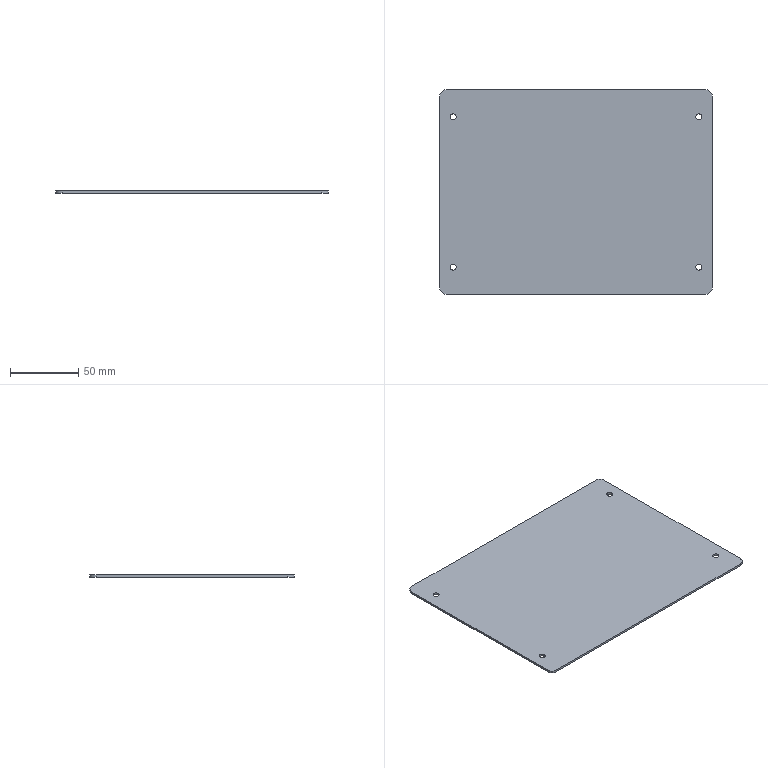Part | SolidWorks | features BaseBody 1 | 1 solid | 18 faces | box 200 x 150 x 1.5 mm | volume 44872 mm3 | cylinder 12 | plane 6 | commonest cylinder face diameters 4.5 x8 10 x4
STEP:
#1=CARTESIAN_POINT('',(-87.75,55.,-1.5));
#2=VERTEX_POINT('',#1);
#3=CARTESIAN_POINT('',(-92.25,55.,-1.5));
#4=VERTEX_POINT('',#3);
#5=CARTESIAN_POINT('',(-90.,55.,-1.5));
#6=DIRECTION('',(0.,0.,-1.));
#7=DIRECTION('',(-1.,0.,0.));
#8=AXIS2_PLACEMENT_3D('',#5,#6,#7);
#9=CIRCLE('',#8,2.25);
#10=EDGE_CURVE('',#2,#4,#9,.T.);
#11=ORIENTED_EDGE('',*,*,#10,.T.);
#12=CARTESIAN_POINT('',(-92.25,55.,0.));
#13=VERTEX_POINT('',#12);
#14=CARTESIAN_POINT('',(-92.25,55.,0.));
#15=DIRECTION('',(0.,0.,1.));
#16=VECTOR('',#15,1000.);
#17=LINE('',#14,#16);
#18=EDGE_CURVE('',#4,#13,#17,.T.);
#19=ORIENTED_EDGE('',*,*,#18,.T.);
#20=CARTESIAN_POINT('',(-87.75,55.,0.));
#21=VERTEX_POINT('',#20);
#22=CARTESIAN_POINT('',(-90.,55.,0.));
#23=DIRECTION('',(0.,0.,1.));
#24=DIRECTION('',(1.,0.,0.));
#25=AXIS2_PLACEMENT_3D('',#22,#23,#24);
#26=CIRCLE('',#25,2.25);
#27=EDGE_CURVE('',#13,#21,#26,.T.);
#28=ORIENTED_EDGE('',*,*,#27,.T.);
#29=CARTESIAN_POINT('',(-87.75,55.,0.));
#30=DIRECTION('',(0.,0.,1.));
#31=VECTOR('',#30,1000.);
#32=LINE('',#29,#31);
#33=EDGE_CURVE('',#2,#21,#32,.T.);
#34=ORIENTED_EDGE('',*,*,#33,.F.);
#35=EDGE_LOOP('',(#11,#19,#28,#34));
#36=FACE_OUTER_BOUND('',#35,.T.);
#37=CARTESIAN_POINT('',(-90.,55.,0.));
#38=DIRECTION('',(0.,0.,1.));
#39=DIRECTION('',(1.,0.,0.));
#40=AXIS2_PLACEMENT_3D('',#37,#38,#39);
#41=CYLINDRICAL_SURFACE('',#40,2.25);
#42=ADVANCED_FACE('',(#36),#41,.F.);
#43=CARTESIAN_POINT('',(92.25,-55.,-1.5));
#44=VERTEX_POINT('',#43);
#45=CARTESIAN_POINT('',(87.75,-55.,-1.5));
#46=VERTEX_POINT('',#45);
#47=CARTESIAN_POINT('',(90.,-55.,-1.5));
#48=DIRECTION('',(0.,0.,-1.));
#49=DIRECTION('',(-1.,0.,0.));
#50=AXIS2_PLACEMENT_3D('',#47,#48,#49);
#51=CIRCLE('',#50,2.25);
#52=EDGE_CURVE('',#44,#46,#51,.T.);
#53=ORIENTED_EDGE('',*,*,#52,.T.);
#54=CARTESIAN_POINT('',(87.75,-55.,0.));
#55=VERTEX_POINT('',#54);
#56=CARTESIAN_POINT('',(87.75,-55.,0.));
#57=DIRECTION('',(0.,0.,1.));
#58=VECTOR('',#57,1000.);
#59=LINE('',#56,#58);
#60=EDGE_CURVE('',#46,#55,#59,.T.);
#61=ORIENTED_EDGE('',*,*,#60,.T.);
#62=CARTESIAN_POINT('',(92.25,-55.,0.));
#63=VERTEX_POINT('',#62);
#64=CARTESIAN_POINT('',(90.,-55.,0.));
#65=DIRECTION('',(0.,0.,1.));
#66=DIRECTION('',(1.,0.,0.));
#67=AXIS2_PLACEMENT_3D('',#64,#65,#66);
#68=CIRCLE('',#67,2.25);
#69=EDGE_CURVE('',#55,#63,#68,.T.);
#70=ORIENTED_EDGE('',*,*,#69,.T.);
#71=CARTESIAN_POINT('',(92.25,-55.,0.));
#72=DIRECTION('',(0.,0.,1.));
#73=VECTOR('',#72,1000.);
#74=LINE('',#71,#73);
#75=EDGE_CURVE('',#44,#63,#74,.T.);
#76=ORIENTED_EDGE('',*,*,#75,.F.);
#77=EDGE_LOOP('',(#53,#61,#70,#76));
#78=FACE_OUTER_BOUND('',#77,.T.);
#79=CARTESIAN_POINT('',(90.,-55.,0.));
#80=DIRECTION('',(0.,0.,1.));
#81=DIRECTION('',(1.,0.,0.));
#82=AXIS2_PLACEMENT_3D('',#79,#80,#81);
#83=CYLINDRICAL_SURFACE('',#82,2.25);
#84=ADVANCED_FACE('',(#78),#83,.F.);
#85=CARTESIAN_POINT('',(-87.75,-55.,-1.5));
#86=VERTEX_POINT('',#85);
#87=CARTESIAN_POINT('',(-92.25,-55.,-1.5));
#88=VERTEX_POINT('',#87);
#89=CARTESIAN_POINT('',(-90.,-55.,-1.5));
#90=DIRECTION('',(0.,0.,-1.));
#91=DIRECTION('',(-1.,0.,0.));
#92=AXIS2_PLACEMENT_3D('',#89,#90,#91);
#93=CIRCLE('',#92,2.25);
#94=EDGE_CURVE('',#86,#88,#93,.T.);
#95=ORIENTED_EDGE('',*,*,#94,.T.);
#96=CARTESIAN_POINT('',(-92.25,-55.,0.));
#97=VERTEX_POINT('',#96);
#98=CARTESIAN_POINT('',(-92.25,-55.,0.));
#99=DIRECTION('',(0.,0.,1.));
#100=VECTOR('',#99,1000.);
#101=LINE('',#98,#100);
#102=EDGE_CURVE('',#88,#97,#101,.T.);
#103=ORIENTED_EDGE('',*,*,#102,.T.);
#104=CARTESIAN_POINT('',(-87.75,-55.,0.));
#105=VERTEX_POINT('',#104);
#106=CARTESIAN_POINT('',(-90.,-55.,0.));
#107=DIRECTION('',(0.,0.,1.));
#108=DIRECTION('',(1.,0.,0.));
#109=AXIS2_PLACEMENT_3D('',#106,#107,#108);
#110=CIRCLE('',#109,2.25);
#111=EDGE_CURVE('',#97,#105,#110,.T.);
#112=ORIENTED_EDGE('',*,*,#111,.T.);
#113=CARTESIAN_POINT('',(-87.75,-55.,0.));
#114=DIRECTION('',(0.,0.,1.));
#115=VECTOR('',#114,1000.);
#116=LINE('',#113,#115);
#117=EDGE_CURVE('',#86,#105,#116,.T.);
#118=ORIENTED_EDGE('',*,*,#117,.F.);
#119=EDGE_LOOP('',(#95,#103,#112,#118));
#120=FACE_OUTER_BOUND('',#119,.T.);
#121=CARTESIAN_POINT('',(-90.,-55.,0.));
#122=DIRECTION('',(0.,0.,1.));
#123=DIRECTION('',(1.,0.,0.));
#124=AXIS2_PLACEMENT_3D('',#121,#122,#123);
#125=CYLINDRICAL_SURFACE('',#124,2.25);
#126=ADVANCED_FACE('',(#120),#125,.F.);
#127=CARTESIAN_POINT('',(92.25,55.,-1.5));
#128=VERTEX_POINT('',#127);
#129=CARTESIAN_POINT('',(87.75,55.,-1.5));
#130=VERTEX_POINT('',#129);
#131=CARTESIAN_POINT('',(90.,55.,-1.5));
#132=DIRECTION('',(0.,0.,-1.));
#133=DIRECTION('',(-1.,0.,0.));
#134=AXIS2_PLACEMENT_3D('',#131,#132,#133);
#135=CIRCLE('',#134,2.25);
#136=EDGE_CURVE('',#128,#130,#135,.T.);
#137=ORIENTED_EDGE('',*,*,#136,.T.);
#138=CARTESIAN_POINT('',(87.75,55.,0.));
#139=VERTEX_POINT('',#138);
#140=CARTESIAN_POINT('',(87.75,55.,0.));
#141=DIRECTION('',(0.,0.,1.));
#142=VECTOR('',#141,1000.);
#143=LINE('',#140,#142);
#144=EDGE_CURVE('',#130,#139,#143,.T.);
#145=ORIENTED_EDGE('',*,*,#144,.T.);
#146=CARTESIAN_POINT('',(92.25,55.,0.));
#147=VERTEX_POINT('',#146);
#148=CARTESIAN_POINT('',(90.,55.,0.));
#149=DIRECTION('',(0.,0.,1.));
#150=DIRECTION('',(1.,0.,0.));
#151=AXIS2_PLACEMENT_3D('',#148,#149,#150);
#152=CIRCLE('',#151,2.25);
#153=EDGE_CURVE('',#139,#147,#152,.T.);
#154=ORIENTED_EDGE('',*,*,#153,.T.);
#155=CARTESIAN_POINT('',(92.25,55.,0.));
#156=DIRECTION('',(0.,0.,1.));
#157=VECTOR('',#156,1000.);
#158=LINE('',#155,#157);
#159=EDGE_CURVE('',#128,#147,#158,.T.);
#160=ORIENTED_EDGE('',*,*,#159,.F.);
#161=EDGE_LOOP('',(#137,#145,#154,#160));
#162=FACE_OUTER_BOUND('',#161,.T.);
#163=CARTESIAN_POINT('',(90.,55.,0.));
#164=DIRECTION('',(0.,0.,1.));
#165=DIRECTION('',(1.,0.,0.));
#166=AXIS2_PLACEMENT_3D('',#163,#164,#165);
#167=CYLINDRICAL_SURFACE('',#166,2.25);
#168=ADVANCED_FACE('',(#162),#167,.F.);
#169=CARTESIAN_POINT('',(-100.,70.,-1.5));
#170=VERTEX_POINT('',#169);
#171=CARTESIAN_POINT('',(-95.,75.,-1.5));
#172=VERTEX_POINT('',#171);
#173=CARTESIAN_POINT('',(-95.,70.,-1.5));
#174=DIRECTION('',(0.,0.,-1.));
#175=DIRECTION('',(-1.,0.,0.));
#176=AXIS2_PLACEMENT_3D('',#173,#174,#175);
#177=CIRCLE('',#176,5.);
#178=EDGE_CURVE('',#170,#172,#177,.T.);
#179=ORIENTED_EDGE('',*,*,#178,.F.);
#180=CARTESIAN_POINT('',(-100.,70.,0.));
#181=VERTEX_POINT('',#180);
#182=CARTESIAN_POINT('',(-100.,70.,-1.5));
#183=DIRECTION('',(0.,0.,-1.));
#184=VECTOR('',#183,1000.);
#185=LINE('',#182,#184);
#186=EDGE_CURVE('',#181,#170,#185,.T.);
#187=ORIENTED_EDGE('',*,*,#186,.F.);
#188=CARTESIAN_POINT('',(-95.,75.,0.));
#189=VERTEX_POINT('',#188);
#190=CARTESIAN_POINT('',(-95.,70.,0.));
#191=DIRECTION('',(0.,0.,1.));
#192=DIRECTION('',(-1.,0.,0.));
#193=AXIS2_PLACEMENT_3D('',#190,#191,#192);
#194=CIRCLE('',#193,5.);
#195=EDGE_CURVE('',#189,#181,#194,.T.);
#196=ORIENTED_EDGE('',*,*,#195,.F.);
#197=CARTESIAN_POINT('',(-95.,75.,-1.5));
#198=DIRECTION('',(0.,0.,1.));
#199=VECTOR('',#198,1000.);
#200=LINE('',#197,#199);
#201=EDGE_CURVE('',#172,#189,#200,.T.);
#202=ORIENTED_EDGE('',*,*,#201,.F.);
#203=EDGE_LOOP('',(#179,#187,#196,#202));
#204=FACE_OUTER_BOUND('',#203,.T.);
#205=CARTESIAN_POINT('',(-95.,70.,-1.5));
#206=DIRECTION('',(0.,0.,1.));
#207=DIRECTION('',(1.,0.,0.));
#208=AXIS2_PLACEMENT_3D('',#205,#206,#207);
#209=CYLINDRICAL_SURFACE('',#208,5.);
#210=ADVANCED_FACE('',(#204),#209,.T.);
#211=CARTESIAN_POINT('',(100.,-70.,-1.5));
#212=VERTEX_POINT('',#211);
#213=CARTESIAN_POINT('',(95.,-75.,-1.5));
#214=VERTEX_POINT('',#213);
#215=CARTESIAN_POINT('',(95.,-70.,-1.5));
#216=DIRECTION('',(0.,0.,-1.));
#217=DIRECTION('',(-1.,0.,0.));
#218=AXIS2_PLACEMENT_3D('',#215,#216,#217);
#219=CIRCLE('',#218,5.);
#220=EDGE_CURVE('',#212,#214,#219,.T.);
#221=ORIENTED_EDGE('',*,*,#220,.F.);
#222=CARTESIAN_POINT('',(100.,-70.,0.));
#223=VERTEX_POINT('',#222);
#224=CARTESIAN_POINT('',(100.,-70.,-1.5));
#225=DIRECTION('',(0.,0.,-1.));
#226=VECTOR('',#225,1000.);
#227=LINE('',#224,#226);
#228=EDGE_CURVE('',#223,#212,#227,.T.);
#229=ORIENTED_EDGE('',*,*,#228,.F.);
#230=CARTESIAN_POINT('',(95.,-75.,0.));
#231=VERTEX_POINT('',#230);
#232=CARTESIAN_POINT('',(95.,-70.,0.));
#233=DIRECTION('',(0.,0.,1.));
#234=DIRECTION('',(-1.,0.,0.));
#235=AXIS2_PLACEMENT_3D('',#232,#233,#234);
#236=CIRCLE('',#235,5.);
#237=EDGE_CURVE('',#231,#223,#236,.T.);
#238=ORIENTED_EDGE('',*,*,#237,.F.);
#239=CARTESIAN_POINT('',(95.,-75.,-1.5));
#240=DIRECTION('',(0.,0.,1.));
#241=VECTOR('',#240,1000.);
#242=LINE('',#239,#241);
#243=EDGE_CURVE('',#214,#231,#242,.T.);
#244=ORIENTED_EDGE('',*,*,#243,.F.);
#245=EDGE_LOOP('',(#221,#229,#238,#244));
#246=FACE_OUTER_BOUND('',#245,.T.);
#247=CARTESIAN_POINT('',(95.,-70.,-1.5));
#248=DIRECTION('',(0.,0.,1.));
#249=DIRECTION('',(1.,0.,0.));
#250=AXIS2_PLACEMENT_3D('',#247,#248,#249);
#251=CYLINDRICAL_SURFACE('',#250,5.);
#252=ADVANCED_FACE('',(#246),#251,.T.);
#253=CARTESIAN_POINT('',(-95.,-75.,-1.5));
#254=VERTEX_POINT('',#253);
#255=CARTESIAN_POINT('',(-100.,-70.,-1.5));
#256=VERTEX_POINT('',#255);
#257=CARTESIAN_POINT('',(-95.,-70.,-1.5));
#258=DIRECTION('',(0.,0.,-1.));
#259=DIRECTION('',(-1.,0.,0.));
#260=AXIS2_PLACEMENT_3D('',#257,#258,#259);
#261=CIRCLE('',#260,5.);
#262=EDGE_CURVE('',#254,#256,#261,.T.);
#263=ORIENTED_EDGE('',*,*,#262,.F.);
#264=CARTESIAN_POINT('',(-95.,-75.,0.));
#265=VERTEX_POINT('',#264);
#266=CARTESIAN_POINT('',(-95.,-75.,-1.5));
#267=DIRECTION('',(0.,0.,-1.));
#268=VECTOR('',#267,1000.);
#269=LINE('',#266,#268);
#270=EDGE_CURVE('',#265,#254,#269,.T.);
#271=ORIENTED_EDGE('',*,*,#270,.F.);
#272=CARTESIAN_POINT('',(-100.,-70.,0.));
#273=VERTEX_POINT('',#272);
#274=CARTESIAN_POINT('',(-95.,-70.,0.));
#275=DIRECTION('',(0.,0.,1.));
#276=DIRECTION('',(-1.,0.,0.));
#277=AXIS2_PLACEMENT_3D('',#274,#275,#276);
#278=CIRCLE('',#277,5.);
#279=EDGE_CURVE('',#273,#265,#278,.T.);
#280=ORIENTED_EDGE('',*,*,#279,.F.);
#281=CARTESIAN_POINT('',(-100.,-70.,-1.5));
#282=DIRECTION('',(0.,0.,1.));
#283=VECTOR('',#282,1000.);
#284=LINE('',#281,#283);
#285=EDGE_CURVE('',#256,#273,#284,.T.);
#286=ORIENTED_EDGE('',*,*,#285,.F.);
#287=EDGE_LOOP('',(#263,#271,#280,#286));
#288=FACE_OUTER_BOUND('',#287,.T.);
#289=CARTESIAN_POINT('',(-95.,-70.,-1.5));
#290=DIRECTION('',(0.,0.,1.));
#291=DIRECTION('',(1.,0.,0.));
#292=AXIS2_PLACEMENT_3D('',#289,#290,#291);
#293=CYLINDRICAL_SURFACE('',#292,5.);
#294=ADVANCED_FACE('',(#288),#293,.T.);
#295=CARTESIAN_POINT('',(95.,75.,-1.5));
#296=VERTEX_POINT('',#295);
#297=CARTESIAN_POINT('',(100.,70.,-1.5));
#298=VERTEX_POINT('',#297);
#299=CARTESIAN_POINT('',(95.,70.,-1.5));
#300=DIRECTION('',(0.,0.,-1.));
#301=DIRECTION('',(-1.,0.,0.));
#302=AXIS2_PLACEMENT_3D('',#299,#300,#301);
#303=CIRCLE('',#302,5.);
#304=EDGE_CURVE('',#296,#298,#303,.T.);
#305=ORIENTED_EDGE('',*,*,#304,.F.);
#306=CARTESIAN_POINT('',(95.,75.,0.));
#307=VERTEX_POINT('',#306);
#308=CARTESIAN_POINT('',(95.,75.,-1.5));
#309=DIRECTION('',(0.,0.,-1.));
#310=VECTOR('',#309,1000.);
#311=LINE('',#308,#310);
#312=EDGE_CURVE('',#307,#296,#311,.T.);
#313=ORIENTED_EDGE('',*,*,#312,.F.);
#314=CARTESIAN_POINT('',(100.,70.,0.));
#315=VERTEX_POINT('',#314);
#316=CARTESIAN_POINT('',(95.,70.,0.));
#317=DIRECTION('',(0.,0.,1.));
#318=DIRECTION('',(-1.,0.,0.));
#319=AXIS2_PLACEMENT_3D('',#316,#317,#318);
#320=CIRCLE('',#319,5.);
#321=EDGE_CURVE('',#315,#307,#320,.T.);
#322=ORIENTED_EDGE('',*,*,#321,.F.);
#323=CARTESIAN_POINT('',(100.,70.,-1.5));
#324=DIRECTION('',(0.,0.,1.));
#325=VECTOR('',#324,1000.);
#326=LINE('',#323,#325);
#327=EDGE_CURVE('',#298,#315,#326,.T.);
#328=ORIENTED_EDGE('',*,*,#327,.F.);
#329=EDGE_LOOP('',(#305,#313,#322,#328));
#330=FACE_OUTER_BOUND('',#329,.T.);
#331=CARTESIAN_POINT('',(95.,70.,-1.5));
#332=DIRECTION('',(0.,0.,1.));
#333=DIRECTION('',(1.,0.,0.));
#334=AXIS2_PLACEMENT_3D('',#331,#332,#333);
#335=CYLINDRICAL_SURFACE('',#334,5.);
#336=ADVANCED_FACE('',(#330),#335,.T.);
#337=ORIENTED_EDGE('',*,*,#136,.F.);
#338=CARTESIAN_POINT('',(90.,55.,-1.5));
#339=DIRECTION('',(0.,0.,-1.));
#340=DIRECTION('',(-1.,0.,0.));
#341=AXIS2_PLACEMENT_3D('',#338,#339,#340);
#342=CIRCLE('',#341,2.25);
#343=EDGE_CURVE('',#130,#128,#342,.T.);
#344=ORIENTED_EDGE('',*,*,#343,.F.);
#345=EDGE_LOOP('',(#337,#344));
#346=FACE_BOUND('',#345,.T.);
#347=ORIENTED_EDGE('',*,*,#94,.F.);
#348=CARTESIAN_POINT('',(-90.,-55.,-1.5));
#349=DIRECTION('',(0.,0.,-1.));
#350=DIRECTION('',(-1.,0.,0.));
#351=AXIS2_PLACEMENT_3D('',#348,#349,#350);
#352=CIRCLE('',#351,2.25);
#353=EDGE_CURVE('',#88,#86,#352,.T.);
#354=ORIENTED_EDGE('',*,*,#353,.F.);
#355=EDGE_LOOP('',(#347,#354));
#356=FACE_BOUND('',#355,.T.);
#357=ORIENTED_EDGE('',*,*,#52,.F.);
#358=CARTESIAN_POINT('',(90.,-55.,-1.5));
#359=DIRECTION('',(0.,0.,-1.));
#360=DIRECTION('',(-1.,0.,0.));
#361=AXIS2_PLACEMENT_3D('',#358,#359,#360);
#362=CIRCLE('',#361,2.25);
#363=EDGE_CURVE('',#46,#44,#362,.T.);
#364=ORIENTED_EDGE('',*,*,#363,.F.);
#365=EDGE_LOOP('',(#357,#364));
#366=FACE_BOUND('',#365,.T.);
#367=ORIENTED_EDGE('',*,*,#10,.F.);
#368=CARTESIAN_POINT('',(-90.,55.,-1.5));
#369=DIRECTION('',(0.,0.,-1.));
#370=DIRECTION('',(-1.,0.,0.));
#371=AXIS2_PLACEMENT_3D('',#368,#369,#370);
#372=CIRCLE('',#371,2.25);
#373=EDGE_CURVE('',#4,#2,#372,.T.);
#374=ORIENTED_EDGE('',*,*,#373,.F.);
#375=EDGE_LOOP('',(#367,#374));
#376=FACE_BOUND('',#375,.T.);
#377=CARTESIAN_POINT('',(-100.,75.,-1.5));
#378=DIRECTION('',(-1.,0.,0.));
#379=VECTOR('',#378,1000.);
#380=LINE('',#377,#379);
#381=EDGE_CURVE('',#296,#172,#380,.T.);
#382=ORIENTED_EDGE('',*,*,#381,.F.);
#383=ORIENTED_EDGE('',*,*,#304,.T.);
#384=CARTESIAN_POINT('',(100.,-75.,-1.5));
#385=DIRECTION('',(0.,1.,0.));
#386=VECTOR('',#385,1000.);
#387=LINE('',#384,#386);
#388=EDGE_CURVE('',#212,#298,#387,.T.);
#389=ORIENTED_EDGE('',*,*,#388,.F.);
#390=ORIENTED_EDGE('',*,*,#220,.T.);
#391=CARTESIAN_POINT('',(-100.,-75.,-1.5));
#392=DIRECTION('',(1.,0.,0.));
#393=VECTOR('',#392,1000.);
#394=LINE('',#391,#393);
#395=EDGE_CURVE('',#254,#214,#394,.T.);
#396=ORIENTED_EDGE('',*,*,#395,.F.);
#397=ORIENTED_EDGE('',*,*,#262,.T.);
#398=CARTESIAN_POINT('',(-100.,-75.,-1.5));
#399=DIRECTION('',(0.,-1.,0.));
#400=VECTOR('',#399,1000.);
#401=LINE('',#398,#400);
#402=EDGE_CURVE('',#170,#256,#401,.T.);
#403=ORIENTED_EDGE('',*,*,#402,.F.);
#404=ORIENTED_EDGE('',*,*,#178,.T.);
#405=EDGE_LOOP('',(#382,#383,#389,#390,#396,#397,#403,#404));
#406=FACE_OUTER_BOUND('',#405,.T.);
#407=CARTESIAN_POINT('',(0.,0.,-1.5));
#408=DIRECTION('',(0.,0.,-1.));
#409=DIRECTION('',(0.,-1.,0.));
#410=AXIS2_PLACEMENT_3D('',#407,#408,#409);
#411=PLANE('',#410);
#412=ADVANCED_FACE('',(#346,#356,#366,#376,#406),#411,.T.);
#413=CARTESIAN_POINT('',(-100.,75.,0.));
#414=DIRECTION('',(-1.,0.,0.));
#415=VECTOR('',#414,1000.);
#416=LINE('',#413,#415);
#417=EDGE_CURVE('',#307,#189,#416,.T.);
#418=ORIENTED_EDGE('',*,*,#417,.F.);
#419=ORIENTED_EDGE('',*,*,#312,.T.);
#420=ORIENTED_EDGE('',*,*,#381,.T.);
#421=ORIENTED_EDGE('',*,*,#201,.T.);
#422=EDGE_LOOP('',(#418,#419,#420,#421));
#423=FACE_OUTER_BOUND('',#422,.T.);
#424=CARTESIAN_POINT('',(-100.,75.,-1.5));
#425=DIRECTION('',(0.,1.,0.));
#426=DIRECTION('',(1.,0.,0.));
#427=AXIS2_PLACEMENT_3D('',#424,#425,#426);
#428=PLANE('',#427);
#429=ADVANCED_FACE('',(#423),#428,.T.);
#430=ORIENTED_EDGE('',*,*,#402,.T.);
#431=ORIENTED_EDGE('',*,*,#285,.T.);
#432=CARTESIAN_POINT('',(-100.,-75.,0.));
#433=DIRECTION('',(0.,-1.,0.));
#434=VECTOR('',#433,1000.);
#435=LINE('',#432,#434);
#436=EDGE_CURVE('',#181,#273,#435,.T.);
#437=ORIENTED_EDGE('',*,*,#436,.F.);
#438=ORIENTED_EDGE('',*,*,#186,.T.);
#439=EDGE_LOOP('',(#430,#431,#437,#438));
#440=FACE_OUTER_BOUND('',#439,.T.);
#441=CARTESIAN_POINT('',(-100.,-75.,-1.5));
#442=DIRECTION('',(-1.,0.,0.));
#443=DIRECTION('',(0.,0.,1.));
#444=AXIS2_PLACEMENT_3D('',#441,#442,#443);
#445=PLANE('',#444);
#446=ADVANCED_FACE('',(#440),#445,.T.);
#447=CARTESIAN_POINT('',(-100.,-75.,0.));
#448=DIRECTION('',(1.,0.,0.));
#449=VECTOR('',#448,1000.);
#450=LINE('',#447,#449);
#451=EDGE_CURVE('',#265,#231,#450,.T.);
#452=ORIENTED_EDGE('',*,*,#451,.F.);
#453=ORIENTED_EDGE('',*,*,#270,.T.);
#454=ORIENTED_EDGE('',*,*,#395,.T.);
#455=ORIENTED_EDGE('',*,*,#243,.T.);
#456=EDGE_LOOP('',(#452,#453,#454,#455));
#457=FACE_OUTER_BOUND('',#456,.T.);
#458=CARTESIAN_POINT('',(-100.,-75.,-1.5));
#459=DIRECTION('',(0.,-1.,0.));
#460=DIRECTION('',(0.,0.,-1.));
#461=AXIS2_PLACEMENT_3D('',#458,#459,#460);
#462=PLANE('',#461);
#463=ADVANCED_FACE('',(#457),#462,.T.);
#464=ORIENTED_EDGE('',*,*,#388,.T.);
#465=ORIENTED_EDGE('',*,*,#327,.T.);
#466=CARTESIAN_POINT('',(100.,-75.,0.));
#467=DIRECTION('',(0.,1.,0.));
#468=VECTOR('',#467,1000.);
#469=LINE('',#466,#468);
#470=EDGE_CURVE('',#223,#315,#469,.T.);
#471=ORIENTED_EDGE('',*,*,#470,.F.);
#472=ORIENTED_EDGE('',*,*,#228,.T.);
#473=EDGE_LOOP('',(#464,#465,#471,#472));
#474=FACE_OUTER_BOUND('',#473,.T.);
#475=CARTESIAN_POINT('',(100.,-75.,-1.5));
#476=DIRECTION('',(1.,0.,0.));
#477=DIRECTION('',(0.,1.,0.));
#478=AXIS2_PLACEMENT_3D('',#475,#476,#477);
#479=PLANE('',#478);
#480=ADVANCED_FACE('',(#474),#479,.T.);
#481=CARTESIAN_POINT('',(-90.,55.,0.));
#482=DIRECTION('',(0.,0.,1.));
#483=DIRECTION('',(1.,0.,0.));
#484=AXIS2_PLACEMENT_3D('',#481,#482,#483);
#485=CIRCLE('',#484,2.25);
#486=EDGE_CURVE('',#21,#13,#485,.T.);
#487=ORIENTED_EDGE('',*,*,#486,.F.);
#488=ORIENTED_EDGE('',*,*,#27,.F.);
#489=EDGE_LOOP('',(#487,#488));
#490=FACE_BOUND('',#489,.T.);
#491=CARTESIAN_POINT('',(90.,55.,0.));
#492=DIRECTION('',(0.,0.,1.));
#493=DIRECTION('',(1.,0.,0.));
#494=AXIS2_PLACEMENT_3D('',#491,#492,#493);
#495=CIRCLE('',#494,2.25);
#496=EDGE_CURVE('',#147,#139,#495,.T.);
#497=ORIENTED_EDGE('',*,*,#496,.F.);
#498=ORIENTED_EDGE('',*,*,#153,.F.);
#499=EDGE_LOOP('',(#497,#498));
#500=FACE_BOUND('',#499,.T.);
#501=CARTESIAN_POINT('',(-90.,-55.,0.));
#502=DIRECTION('',(0.,0.,1.));
#503=DIRECTION('',(1.,0.,0.));
#504=AXIS2_PLACEMENT_3D('',#501,#502,#503);
#505=CIRCLE('',#504,2.25);
#506=EDGE_CURVE('',#105,#97,#505,.T.);
#507=ORIENTED_EDGE('',*,*,#506,.F.);
#508=ORIENTED_EDGE('',*,*,#111,.F.);
#509=EDGE_LOOP('',(#507,#508));
#510=FACE_BOUND('',#509,.T.);
#511=CARTESIAN_POINT('',(90.,-55.,0.));
#512=DIRECTION('',(0.,0.,1.));
#513=DIRECTION('',(1.,0.,0.));
#514=AXIS2_PLACEMENT_3D('',#511,#512,#513);
#515=CIRCLE('',#514,2.25);
#516=EDGE_CURVE('',#63,#55,#515,.T.);
#517=ORIENTED_EDGE('',*,*,#516,.F.);
#518=ORIENTED_EDGE('',*,*,#69,.F.);
#519=EDGE_LOOP('',(#517,#518));
#520=FACE_BOUND('',#519,.T.);
#521=ORIENTED_EDGE('',*,*,#470,.T.);
#522=ORIENTED_EDGE('',*,*,#321,.T.);
#523=ORIENTED_EDGE('',*,*,#417,.T.);
#524=ORIENTED_EDGE('',*,*,#195,.T.);
#525=ORIENTED_EDGE('',*,*,#436,.T.);
#526=ORIENTED_EDGE('',*,*,#279,.T.);
#527=ORIENTED_EDGE('',*,*,#451,.T.);
#528=ORIENTED_EDGE('',*,*,#237,.T.);
#529=EDGE_LOOP('',(#521,#522,#523,#524,#525,#526,#527,#528));
#530=FACE_OUTER_BOUND('',#529,.T.);
#531=CARTESIAN_POINT('',(0.,0.,0.));
#532=DIRECTION('',(0.,0.,-1.));
#533=DIRECTION('',(0.,-1.,0.));
#534=AXIS2_PLACEMENT_3D('',#531,#532,#533);
#535=PLANE('',#534);
#536=ADVANCED_FACE('',(#490,#500,#510,#520,#530),#535,.F.);
#537=ORIENTED_EDGE('',*,*,#144,.F.);
#538=ORIENTED_EDGE('',*,*,#343,.T.);
#539=ORIENTED_EDGE('',*,*,#159,.T.);
#540=ORIENTED_EDGE('',*,*,#496,.T.);
#541=EDGE_LOOP('',(#537,#538,#539,#540));
#542=FACE_OUTER_BOUND('',#541,.T.);
#543=CARTESIAN_POINT('',(90.,55.,0.));
#544=DIRECTION('',(0.,0.,1.));
#545=DIRECTION('',(1.,0.,0.));
#546=AXIS2_PLACEMENT_3D('',#543,#544,#545);
#547=CYLINDRICAL_SURFACE('',#546,2.25);
#548=ADVANCED_FACE('',(#542),#547,.F.);
#549=ORIENTED_EDGE('',*,*,#102,.F.);
#550=ORIENTED_EDGE('',*,*,#353,.T.);
#551=ORIENTED_EDGE('',*,*,#117,.T.);
#552=ORIENTED_EDGE('',*,*,#506,.T.);
#553=EDGE_LOOP('',(#549,#550,#551,#552));
#554=FACE_OUTER_BOUND('',#553,.T.);
#555=CARTESIAN_POINT('',(-90.,-55.,0.));
#556=DIRECTION('',(0.,0.,1.));
#557=DIRECTION('',(1.,0.,0.));
#558=AXIS2_PLACEMENT_3D('',#555,#556,#557);
#559=CYLINDRICAL_SURFACE('',#558,2.25);
#560=ADVANCED_FACE('',(#554),#559,.F.);
#561=ORIENTED_EDGE('',*,*,#60,.F.);
#562=ORIENTED_EDGE('',*,*,#363,.T.);
#563=ORIENTED_EDGE('',*,*,#75,.T.);
#564=ORIENTED_EDGE('',*,*,#516,.T.);
#565=EDGE_LOOP('',(#561,#562,#563,#564));
#566=FACE_OUTER_BOUND('',#565,.T.);
#567=CARTESIAN_POINT('',(90.,-55.,0.));
#568=DIRECTION('',(0.,0.,1.));
#569=DIRECTION('',(1.,0.,0.));
#570=AXIS2_PLACEMENT_3D('',#567,#568,#569);
#571=CYLINDRICAL_SURFACE('',#570,2.25);
#572=ADVANCED_FACE('',(#566),#571,.F.);
#573=ORIENTED_EDGE('',*,*,#18,.F.);
#574=ORIENTED_EDGE('',*,*,#373,.T.);
#575=ORIENTED_EDGE('',*,*,#33,.T.);
#576=ORIENTED_EDGE('',*,*,#486,.T.);
#577=EDGE_LOOP('',(#573,#574,#575,#576));
#578=FACE_OUTER_BOUND('',#577,.T.);
#579=CARTESIAN_POINT('',(-90.,55.,0.));
#580=DIRECTION('',(0.,0.,1.));
#581=DIRECTION('',(1.,0.,0.));
#582=AXIS2_PLACEMENT_3D('',#579,#580,#581);
#583=CYLINDRICAL_SURFACE('',#582,2.25);
#584=ADVANCED_FACE('',(#578),#583,.F.);
#585=CLOSED_SHELL('',(#42,#84,#126,#168,#210,#252,#294,#336,#412,#429,#446,#463,#480,#536,#548,#560,#572,#584));
#586=MANIFOLD_SOLID_BREP('',#585);
#587=CARTESIAN_POINT('',(0.,0.,0.));
#588=DIRECTION('',(0.,0.,1.));
#589=DIRECTION('',(1.,0.,0.));
#590=AXIS2_PLACEMENT_3D('',#587,#588,#589);
#591=(LENGTH_UNIT()NAMED_UNIT(*)SI_UNIT(.MILLI.,.METRE.));
#592=UNCERTAINTY_MEASURE_WITH_UNIT(LENGTH_MEASURE(0.00001),#591,'','');
#593=(NAMED_UNIT(*)PLANE_ANGLE_UNIT()SI_UNIT($,.RADIAN.));
#594=(NAMED_UNIT(*)SI_UNIT($,.STERADIAN.)SOLID_ANGLE_UNIT());
#595=(GEOMETRIC_REPRESENTATION_CONTEXT(3)GLOBAL_UNCERTAINTY_ASSIGNED_CONTEXT((#592))GLOBAL_UNIT_ASSIGNED_CONTEXT((#591,#593,#594))REPRESENTATION_CONTEXT('',''));
#596=ADVANCED_BREP_SHAPE_REPRESENTATION('',(#586,#590),#595);